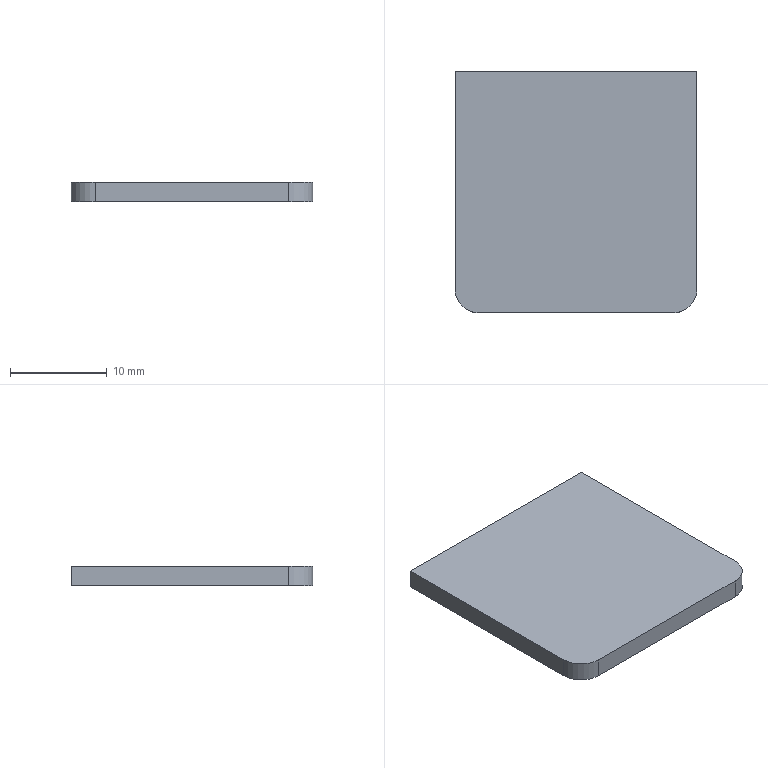Part | STEP file | 5090507 | 1 solid | 8 faces | box 25 x 25 x 2 mm | volume 1245 mm3 | plane 6 | cylinder 2 | commonest cylinder face diameters 5 x2
STEP:
#1=CARTESIAN_POINT('',(0.,0.,0.));
#2=DIRECTION('',(0.,0.,1.));
#3=DIRECTION('',(1.,0.,0.));
#4=AXIS2_PLACEMENT_3D('',#1,#2,#3);
#5=CARTESIAN_POINT('',(-12.5,12.5,0.));
#6=VERTEX_POINT('',#5);
#7=CARTESIAN_POINT('',(-12.5,-10.,0.));
#8=VERTEX_POINT('',#7);
#9=CARTESIAN_POINT('',(-12.5,12.5,0.));
#10=DIRECTION('',(0.,-1.,0.));
#11=VECTOR('',#10,1.);
#12=LINE('',#9,#11);
#13=CARTESIAN_POINT('',(-12.5,12.5,2.));
#14=DIRECTION('',(1.,0.,0.));
#15=DIRECTION('',(0.,1.,0.));
#16=AXIS2_PLACEMENT_3D('',#13,#14,#15);
#17=PLANE('',#16);
#18=CARTESIAN_POINT('',(0.,-2.));
#19=DIRECTION('',(-1.,0.));
#20=VECTOR('',#19,1.);
#21=LINE('',#18,#20);
#22=(GEOMETRIC_REPRESENTATION_CONTEXT(2)PARAMETRIC_REPRESENTATION_CONTEXT()REPRESENTATION_CONTEXT('',''));
#23=DEFINITIONAL_REPRESENTATION('',(#21),#22);
#24=PCURVE('',#17,#23);
#25=CARTESIAN_POINT('',(-10.,-10.,0.));
#26=DIRECTION('',(0.,0.,-1.));
#27=DIRECTION('',(-1.,0.,0.));
#28=AXIS2_PLACEMENT_3D('',#25,#26,#27);
#29=PLANE('',#28);
#30=CARTESIAN_POINT('',(2.5,22.5));
#31=DIRECTION('',(0.,-1.));
#32=VECTOR('',#31,1.);
#33=LINE('',#30,#32);
#34=(GEOMETRIC_REPRESENTATION_CONTEXT(2)PARAMETRIC_REPRESENTATION_CONTEXT()REPRESENTATION_CONTEXT('',''));
#35=DEFINITIONAL_REPRESENTATION('',(#33),#34);
#36=PCURVE('',#29,#35);
#37=SURFACE_CURVE('',#12,(#24,#36),.PCURVE_S1.);
#38=EDGE_CURVE('',#6,#8,#37,.T.);
#39=ORIENTED_EDGE('',*,*,#38,.T.);
#40=CARTESIAN_POINT('',(-12.5,-10.,2.));
#41=VERTEX_POINT('',#40);
#42=CARTESIAN_POINT('',(-12.5,-10.,2.));
#43=DIRECTION('',(0.,0.,-1.));
#44=VECTOR('',#43,1.);
#45=LINE('',#42,#44);
#46=CARTESIAN_POINT('',(-22.5,0.));
#47=DIRECTION('',(0.,-1.));
#48=VECTOR('',#47,1.);
#49=LINE('',#46,#48);
#50=(GEOMETRIC_REPRESENTATION_CONTEXT(2)PARAMETRIC_REPRESENTATION_CONTEXT()REPRESENTATION_CONTEXT('',''));
#51=DEFINITIONAL_REPRESENTATION('',(#49),#50);
#52=PCURVE('',#17,#51);
#53=CARTESIAN_POINT('',(-10.,-10.,2.));
#54=DIRECTION('',(0.,0.,-1.));
#55=DIRECTION('',(-1.,0.,0.));
#56=AXIS2_PLACEMENT_3D('',#53,#54,#55);
#57=CYLINDRICAL_SURFACE('',#56,2.5);
#58=CARTESIAN_POINT('',(6.283,0.));
#59=DIRECTION('',(0.,1.));
#60=VECTOR('',#59,1.);
#61=LINE('',#58,#60);
#62=(GEOMETRIC_REPRESENTATION_CONTEXT(2)PARAMETRIC_REPRESENTATION_CONTEXT()REPRESENTATION_CONTEXT('',''));
#63=DEFINITIONAL_REPRESENTATION('',(#61),#62);
#64=PCURVE('',#57,#63);
#65=SURFACE_CURVE('',#45,(#52,#64),.PCURVE_S1.);
#66=EDGE_CURVE('',#41,#8,#65,.T.);
#67=ORIENTED_EDGE('',*,*,#66,.F.);
#68=CARTESIAN_POINT('',(-12.5,12.5,2.));
#69=VERTEX_POINT('',#68);
#70=CARTESIAN_POINT('',(-12.5,12.5,2.));
#71=DIRECTION('',(0.,-1.,0.));
#72=VECTOR('',#71,1.);
#73=LINE('',#70,#72);
#74=CARTESIAN_POINT('',(0.,0.));
#75=DIRECTION('',(-1.,0.));
#76=VECTOR('',#75,1.);
#77=LINE('',#74,#76);
#78=(GEOMETRIC_REPRESENTATION_CONTEXT(2)PARAMETRIC_REPRESENTATION_CONTEXT()REPRESENTATION_CONTEXT('',''));
#79=DEFINITIONAL_REPRESENTATION('',(#77),#78);
#80=PCURVE('',#17,#79);
#81=CARTESIAN_POINT('',(-10.,-10.,2.));
#82=DIRECTION('',(0.,0.,-1.));
#83=DIRECTION('',(-1.,0.,0.));
#84=AXIS2_PLACEMENT_3D('',#81,#82,#83);
#85=PLANE('',#84);
#86=CARTESIAN_POINT('',(2.5,22.5));
#87=DIRECTION('',(0.,-1.));
#88=VECTOR('',#87,1.);
#89=LINE('',#86,#88);
#90=(GEOMETRIC_REPRESENTATION_CONTEXT(2)PARAMETRIC_REPRESENTATION_CONTEXT()REPRESENTATION_CONTEXT('',''));
#91=DEFINITIONAL_REPRESENTATION('',(#89),#90);
#92=PCURVE('',#85,#91);
#93=SURFACE_CURVE('',#73,(#80,#92),.PCURVE_S1.);
#94=EDGE_CURVE('',#69,#41,#93,.T.);
#95=ORIENTED_EDGE('',*,*,#94,.F.);
#96=CARTESIAN_POINT('',(-12.5,12.5,2.));
#97=DIRECTION('',(0.,0.,-1.));
#98=VECTOR('',#97,1.);
#99=LINE('',#96,#98);
#100=CARTESIAN_POINT('',(0.,0.));
#101=DIRECTION('',(0.,-1.));
#102=VECTOR('',#101,1.);
#103=LINE('',#100,#102);
#104=(GEOMETRIC_REPRESENTATION_CONTEXT(2)PARAMETRIC_REPRESENTATION_CONTEXT()REPRESENTATION_CONTEXT('',''));
#105=DEFINITIONAL_REPRESENTATION('',(#103),#104);
#106=PCURVE('',#17,#105);
#107=CARTESIAN_POINT('',(-12.5,12.5,2.));
#108=DIRECTION('',(0.,-1.,0.));
#109=DIRECTION('',(0.,0.,-1.));
#110=AXIS2_PLACEMENT_3D('',#107,#108,#109);
#111=PLANE('',#110);
#112=CARTESIAN_POINT('',(0.,0.));
#113=DIRECTION('',(1.,0.));
#114=VECTOR('',#113,1.);
#115=LINE('',#112,#114);
#116=(GEOMETRIC_REPRESENTATION_CONTEXT(2)PARAMETRIC_REPRESENTATION_CONTEXT()REPRESENTATION_CONTEXT('',''));
#117=DEFINITIONAL_REPRESENTATION('',(#115),#116);
#118=PCURVE('',#111,#117);
#119=SURFACE_CURVE('',#99,(#106,#118),.PCURVE_S1.);
#120=EDGE_CURVE('',#69,#6,#119,.T.);
#121=ORIENTED_EDGE('',*,*,#120,.T.);
#122=EDGE_LOOP('',(#39,#67,#95,#121));
#123=FACE_BOUND('',#122,.T.);
#124=ADVANCED_FACE('',(#123),#17,.F.);
#125=CARTESIAN_POINT('',(-10.,-12.5,0.));
#126=VERTEX_POINT('',#125);
#127=CARTESIAN_POINT('',(-10.,-10.,0.));
#128=DIRECTION('',(0.,0.,1.));
#129=DIRECTION('',(-1.,0.,0.));
#130=AXIS2_PLACEMENT_3D('',#127,#128,#129);
#131=CIRCLE('',#130,2.5);
#132=CARTESIAN_POINT('',(6.283,2.));
#133=DIRECTION('',(-1.,0.));
#134=VECTOR('',#133,1.);
#135=LINE('',#132,#134);
#136=(GEOMETRIC_REPRESENTATION_CONTEXT(2)PARAMETRIC_REPRESENTATION_CONTEXT()REPRESENTATION_CONTEXT('',''));
#137=DEFINITIONAL_REPRESENTATION('',(#135),#136);
#138=PCURVE('',#57,#137);
#139=CARTESIAN_POINT('',(2.5,0.));
#140=CARTESIAN_POINT('',(2.5,-4.33));
#141=CARTESIAN_POINT('',(-1.25,-2.165));
#142=CARTESIAN_POINT('',(-5.,0.));
#143=CARTESIAN_POINT('',(-1.25,2.165));
#144=CARTESIAN_POINT('',(2.5,4.33));
#145=CARTESIAN_POINT('',(2.5,0.));
#146=(BOUNDED_CURVE()B_SPLINE_CURVE(2,(#139,#140,#141,#142,#143,#144,#145),.UNSPECIFIED.,.T.,.F.)B_SPLINE_CURVE_WITH_KNOTS((1,2,2,2,2,1),(-2.094,0.,2.094,4.189,6.283,8.378),.UNSPECIFIED.)CURVE()GEOMETRIC_REPRESENTATION_ITEM()RATIONAL_B_SPLINE_CURVE((1.,0.5,1.,0.5,1.,0.5,1.))REPRESENTATION_ITEM(''));
#147=(GEOMETRIC_REPRESENTATION_CONTEXT(2)PARAMETRIC_REPRESENTATION_CONTEXT()REPRESENTATION_CONTEXT('',''));
#148=DEFINITIONAL_REPRESENTATION('',(#146),#147);
#149=PCURVE('',#29,#148);
#150=SURFACE_CURVE('',#131,(#138,#149),.PCURVE_S1.);
#151=EDGE_CURVE('',#8,#126,#150,.T.);
#152=ORIENTED_EDGE('',*,*,#151,.T.);
#153=CARTESIAN_POINT('',(-10.,-12.5,2.));
#154=VERTEX_POINT('',#153);
#155=CARTESIAN_POINT('',(-10.,-12.5,2.));
#156=DIRECTION('',(0.,0.,-1.));
#157=VECTOR('',#156,1.);
#158=LINE('',#155,#157);
#159=CARTESIAN_POINT('',(4.712,0.));
#160=DIRECTION('',(0.,1.));
#161=VECTOR('',#160,1.);
#162=LINE('',#159,#161);
#163=(GEOMETRIC_REPRESENTATION_CONTEXT(2)PARAMETRIC_REPRESENTATION_CONTEXT()REPRESENTATION_CONTEXT('',''));
#164=DEFINITIONAL_REPRESENTATION('',(#162),#163);
#165=PCURVE('',#57,#164);
#166=CARTESIAN_POINT('',(-10.,-12.5,2.));
#167=DIRECTION('',(0.,1.,0.));
#168=DIRECTION('',(0.,0.,1.));
#169=AXIS2_PLACEMENT_3D('',#166,#167,#168);
#170=PLANE('',#169);
#171=CARTESIAN_POINT('',(0.,0.));
#172=DIRECTION('',(-1.,0.));
#173=VECTOR('',#172,1.);
#174=LINE('',#171,#173);
#175=(GEOMETRIC_REPRESENTATION_CONTEXT(2)PARAMETRIC_REPRESENTATION_CONTEXT()REPRESENTATION_CONTEXT('',''));
#176=DEFINITIONAL_REPRESENTATION('',(#174),#175);
#177=PCURVE('',#170,#176);
#178=SURFACE_CURVE('',#158,(#165,#177),.PCURVE_S1.);
#179=EDGE_CURVE('',#154,#126,#178,.T.);
#180=ORIENTED_EDGE('',*,*,#179,.F.);
#181=CARTESIAN_POINT('',(-10.,-10.,2.));
#182=DIRECTION('',(0.,0.,1.));
#183=DIRECTION('',(-1.,0.,0.));
#184=AXIS2_PLACEMENT_3D('',#181,#182,#183);
#185=CIRCLE('',#184,2.5);
#186=CARTESIAN_POINT('',(6.283,0.));
#187=DIRECTION('',(-1.,0.));
#188=VECTOR('',#187,1.);
#189=LINE('',#186,#188);
#190=(GEOMETRIC_REPRESENTATION_CONTEXT(2)PARAMETRIC_REPRESENTATION_CONTEXT()REPRESENTATION_CONTEXT('',''));
#191=DEFINITIONAL_REPRESENTATION('',(#189),#190);
#192=PCURVE('',#57,#191);
#193=CARTESIAN_POINT('',(2.5,0.));
#194=CARTESIAN_POINT('',(2.5,-4.33));
#195=CARTESIAN_POINT('',(-1.25,-2.165));
#196=CARTESIAN_POINT('',(-5.,0.));
#197=CARTESIAN_POINT('',(-1.25,2.165));
#198=CARTESIAN_POINT('',(2.5,4.33));
#199=CARTESIAN_POINT('',(2.5,0.));
#200=(BOUNDED_CURVE()B_SPLINE_CURVE(2,(#193,#194,#195,#196,#197,#198,#199),.UNSPECIFIED.,.T.,.F.)B_SPLINE_CURVE_WITH_KNOTS((1,2,2,2,2,1),(-2.094,0.,2.094,4.189,6.283,8.378),.UNSPECIFIED.)CURVE()GEOMETRIC_REPRESENTATION_ITEM()RATIONAL_B_SPLINE_CURVE((1.,0.5,1.,0.5,1.,0.5,1.))REPRESENTATION_ITEM(''));
#201=(GEOMETRIC_REPRESENTATION_CONTEXT(2)PARAMETRIC_REPRESENTATION_CONTEXT()REPRESENTATION_CONTEXT('',''));
#202=DEFINITIONAL_REPRESENTATION('',(#200),#201);
#203=PCURVE('',#85,#202);
#204=SURFACE_CURVE('',#185,(#192,#203),.PCURVE_S1.);
#205=EDGE_CURVE('',#41,#154,#204,.T.);
#206=ORIENTED_EDGE('',*,*,#205,.F.);
#207=ORIENTED_EDGE('',*,*,#66,.T.);
#208=EDGE_LOOP('',(#152,#180,#206,#207));
#209=FACE_BOUND('',#208,.T.);
#210=ADVANCED_FACE('',(#209),#57,.T.);
#211=CARTESIAN_POINT('',(10.,-12.5,0.));
#212=VERTEX_POINT('',#211);
#213=CARTESIAN_POINT('',(-10.,-12.5,0.));
#214=DIRECTION('',(1.,0.,0.));
#215=VECTOR('',#214,1.);
#216=LINE('',#213,#215);
#217=CARTESIAN_POINT('',(-2.,0.));
#218=DIRECTION('',(0.,1.));
#219=VECTOR('',#218,1.);
#220=LINE('',#217,#219);
#221=(GEOMETRIC_REPRESENTATION_CONTEXT(2)PARAMETRIC_REPRESENTATION_CONTEXT()REPRESENTATION_CONTEXT('',''));
#222=DEFINITIONAL_REPRESENTATION('',(#220),#221);
#223=PCURVE('',#170,#222);
#224=CARTESIAN_POINT('',(0.,-2.5));
#225=DIRECTION('',(-1.,0.));
#226=VECTOR('',#225,1.);
#227=LINE('',#224,#226);
#228=(GEOMETRIC_REPRESENTATION_CONTEXT(2)PARAMETRIC_REPRESENTATION_CONTEXT()REPRESENTATION_CONTEXT('',''));
#229=DEFINITIONAL_REPRESENTATION('',(#227),#228);
#230=PCURVE('',#29,#229);
#231=SURFACE_CURVE('',#216,(#223,#230),.PCURVE_S1.);
#232=EDGE_CURVE('',#126,#212,#231,.T.);
#233=ORIENTED_EDGE('',*,*,#232,.T.);
#234=CARTESIAN_POINT('',(10.,-12.5,2.));
#235=VERTEX_POINT('',#234);
#236=CARTESIAN_POINT('',(10.,-12.5,2.));
#237=DIRECTION('',(0.,0.,-1.));
#238=VECTOR('',#237,1.);
#239=LINE('',#236,#238);
#240=CARTESIAN_POINT('',(0.,20.));
#241=DIRECTION('',(-1.,0.));
#242=VECTOR('',#241,1.);
#243=LINE('',#240,#242);
#244=(GEOMETRIC_REPRESENTATION_CONTEXT(2)PARAMETRIC_REPRESENTATION_CONTEXT()REPRESENTATION_CONTEXT('',''));
#245=DEFINITIONAL_REPRESENTATION('',(#243),#244);
#246=PCURVE('',#170,#245);
#247=CARTESIAN_POINT('',(10.,-10.,2.));
#248=DIRECTION('',(0.,0.,-1.));
#249=DIRECTION('',(-1.,0.,0.));
#250=AXIS2_PLACEMENT_3D('',#247,#248,#249);
#251=CYLINDRICAL_SURFACE('',#250,2.5);
#252=CARTESIAN_POINT('',(4.712,0.));
#253=DIRECTION('',(0.,1.));
#254=VECTOR('',#253,1.);
#255=LINE('',#252,#254);
#256=(GEOMETRIC_REPRESENTATION_CONTEXT(2)PARAMETRIC_REPRESENTATION_CONTEXT()REPRESENTATION_CONTEXT('',''));
#257=DEFINITIONAL_REPRESENTATION('',(#255),#256);
#258=PCURVE('',#251,#257);
#259=SURFACE_CURVE('',#239,(#246,#258),.PCURVE_S1.);
#260=EDGE_CURVE('',#235,#212,#259,.T.);
#261=ORIENTED_EDGE('',*,*,#260,.F.);
#262=CARTESIAN_POINT('',(-10.,-12.5,2.));
#263=DIRECTION('',(1.,0.,0.));
#264=VECTOR('',#263,1.);
#265=LINE('',#262,#264);
#266=CARTESIAN_POINT('',(0.,0.));
#267=DIRECTION('',(0.,1.));
#268=VECTOR('',#267,1.);
#269=LINE('',#266,#268);
#270=(GEOMETRIC_REPRESENTATION_CONTEXT(2)PARAMETRIC_REPRESENTATION_CONTEXT()REPRESENTATION_CONTEXT('',''));
#271=DEFINITIONAL_REPRESENTATION('',(#269),#270);
#272=PCURVE('',#170,#271);
#273=CARTESIAN_POINT('',(0.,-2.5));
#274=DIRECTION('',(-1.,0.));
#275=VECTOR('',#274,1.);
#276=LINE('',#273,#275);
#277=(GEOMETRIC_REPRESENTATION_CONTEXT(2)PARAMETRIC_REPRESENTATION_CONTEXT()REPRESENTATION_CONTEXT('',''));
#278=DEFINITIONAL_REPRESENTATION('',(#276),#277);
#279=PCURVE('',#85,#278);
#280=SURFACE_CURVE('',#265,(#272,#279),.PCURVE_S1.);
#281=EDGE_CURVE('',#154,#235,#280,.T.);
#282=ORIENTED_EDGE('',*,*,#281,.F.);
#283=ORIENTED_EDGE('',*,*,#179,.T.);
#284=EDGE_LOOP('',(#233,#261,#282,#283));
#285=FACE_BOUND('',#284,.T.);
#286=ADVANCED_FACE('',(#285),#170,.F.);
#287=CARTESIAN_POINT('',(12.5,-10.,0.));
#288=VERTEX_POINT('',#287);
#289=CARTESIAN_POINT('',(10.,-10.,0.));
#290=DIRECTION('',(0.,0.,1.));
#291=DIRECTION('',(-1.,0.,0.));
#292=AXIS2_PLACEMENT_3D('',#289,#290,#291);
#293=CIRCLE('',#292,2.5);
#294=CARTESIAN_POINT('',(6.283,2.));
#295=DIRECTION('',(-1.,0.));
#296=VECTOR('',#295,1.);
#297=LINE('',#294,#296);
#298=(GEOMETRIC_REPRESENTATION_CONTEXT(2)PARAMETRIC_REPRESENTATION_CONTEXT()REPRESENTATION_CONTEXT('',''));
#299=DEFINITIONAL_REPRESENTATION('',(#297),#298);
#300=PCURVE('',#251,#299);
#301=CARTESIAN_POINT('',(-17.5,0.));
#302=CARTESIAN_POINT('',(-17.5,-4.33));
#303=CARTESIAN_POINT('',(-21.25,-2.165));
#304=CARTESIAN_POINT('',(-25.,0.));
#305=CARTESIAN_POINT('',(-21.25,2.165));
#306=CARTESIAN_POINT('',(-17.5,4.33));
#307=CARTESIAN_POINT('',(-17.5,0.));
#308=(BOUNDED_CURVE()B_SPLINE_CURVE(2,(#301,#302,#303,#304,#305,#306,#307),.UNSPECIFIED.,.T.,.F.)B_SPLINE_CURVE_WITH_KNOTS((1,2,2,2,2,1),(-2.094,0.,2.094,4.189,6.283,8.378),.UNSPECIFIED.)CURVE()GEOMETRIC_REPRESENTATION_ITEM()RATIONAL_B_SPLINE_CURVE((1.,0.5,1.,0.5,1.,0.5,1.))REPRESENTATION_ITEM(''));
#309=(GEOMETRIC_REPRESENTATION_CONTEXT(2)PARAMETRIC_REPRESENTATION_CONTEXT()REPRESENTATION_CONTEXT('',''));
#310=DEFINITIONAL_REPRESENTATION('',(#308),#309);
#311=PCURVE('',#29,#310);
#312=SURFACE_CURVE('',#293,(#300,#311),.PCURVE_S1.);
#313=EDGE_CURVE('',#212,#288,#312,.T.);
#314=ORIENTED_EDGE('',*,*,#313,.T.);
#315=CARTESIAN_POINT('',(12.5,-10.,2.));
#316=VERTEX_POINT('',#315);
#317=CARTESIAN_POINT('',(12.5,-10.,2.));
#318=DIRECTION('',(0.,0.,-1.));
#319=VECTOR('',#318,1.);
#320=LINE('',#317,#319);
#321=CARTESIAN_POINT('',(3.142,0.));
#322=DIRECTION('',(0.,1.));
#323=VECTOR('',#322,1.);
#324=LINE('',#321,#323);
#325=(GEOMETRIC_REPRESENTATION_CONTEXT(2)PARAMETRIC_REPRESENTATION_CONTEXT()REPRESENTATION_CONTEXT('',''));
#326=DEFINITIONAL_REPRESENTATION('',(#324),#325);
#327=PCURVE('',#251,#326);
#328=CARTESIAN_POINT('',(12.5,12.5,2.));
#329=DIRECTION('',(-1.,0.,0.));
#330=DIRECTION('',(0.,-1.,0.));
#331=AXIS2_PLACEMENT_3D('',#328,#329,#330);
#332=PLANE('',#331);
#333=CARTESIAN_POINT('',(22.5,0.));
#334=DIRECTION('',(0.,-1.));
#335=VECTOR('',#334,1.);
#336=LINE('',#333,#335);
#337=(GEOMETRIC_REPRESENTATION_CONTEXT(2)PARAMETRIC_REPRESENTATION_CONTEXT()REPRESENTATION_CONTEXT('',''));
#338=DEFINITIONAL_REPRESENTATION('',(#336),#337);
#339=PCURVE('',#332,#338);
#340=SURFACE_CURVE('',#320,(#327,#339),.PCURVE_S1.);
#341=EDGE_CURVE('',#316,#288,#340,.T.);
#342=ORIENTED_EDGE('',*,*,#341,.F.);
#343=CARTESIAN_POINT('',(10.,-10.,2.));
#344=DIRECTION('',(0.,0.,1.));
#345=DIRECTION('',(-1.,0.,0.));
#346=AXIS2_PLACEMENT_3D('',#343,#344,#345);
#347=CIRCLE('',#346,2.5);
#348=CARTESIAN_POINT('',(6.283,0.));
#349=DIRECTION('',(-1.,0.));
#350=VECTOR('',#349,1.);
#351=LINE('',#348,#350);
#352=(GEOMETRIC_REPRESENTATION_CONTEXT(2)PARAMETRIC_REPRESENTATION_CONTEXT()REPRESENTATION_CONTEXT('',''));
#353=DEFINITIONAL_REPRESENTATION('',(#351),#352);
#354=PCURVE('',#251,#353);
#355=CARTESIAN_POINT('',(-17.5,0.));
#356=CARTESIAN_POINT('',(-17.5,-4.33));
#357=CARTESIAN_POINT('',(-21.25,-2.165));
#358=CARTESIAN_POINT('',(-25.,0.));
#359=CARTESIAN_POINT('',(-21.25,2.165));
#360=CARTESIAN_POINT('',(-17.5,4.33));
#361=CARTESIAN_POINT('',(-17.5,0.));
#362=(BOUNDED_CURVE()B_SPLINE_CURVE(2,(#355,#356,#357,#358,#359,#360,#361),.UNSPECIFIED.,.T.,.F.)B_SPLINE_CURVE_WITH_KNOTS((1,2,2,2,2,1),(-2.094,0.,2.094,4.189,6.283,8.378),.UNSPECIFIED.)CURVE()GEOMETRIC_REPRESENTATION_ITEM()RATIONAL_B_SPLINE_CURVE((1.,0.5,1.,0.5,1.,0.5,1.))REPRESENTATION_ITEM(''));
#363=(GEOMETRIC_REPRESENTATION_CONTEXT(2)PARAMETRIC_REPRESENTATION_CONTEXT()REPRESENTATION_CONTEXT('',''));
#364=DEFINITIONAL_REPRESENTATION('',(#362),#363);
#365=PCURVE('',#85,#364);
#366=SURFACE_CURVE('',#347,(#354,#365),.PCURVE_S1.);
#367=EDGE_CURVE('',#235,#316,#366,.T.);
#368=ORIENTED_EDGE('',*,*,#367,.F.);
#369=ORIENTED_EDGE('',*,*,#260,.T.);
#370=EDGE_LOOP('',(#314,#342,#368,#369));
#371=FACE_BOUND('',#370,.T.);
#372=ADVANCED_FACE('',(#371),#251,.T.);
#373=CARTESIAN_POINT('',(12.5,12.5,0.));
#374=VERTEX_POINT('',#373);
#375=CARTESIAN_POINT('',(12.5,12.5,0.));
#376=DIRECTION('',(0.,1.,0.));
#377=VECTOR('',#376,1.);
#378=LINE('',#375,#377);
#379=CARTESIAN_POINT('',(0.,-2.));
#380=DIRECTION('',(-1.,0.));
#381=VECTOR('',#380,1.);
#382=LINE('',#379,#381);
#383=(GEOMETRIC_REPRESENTATION_CONTEXT(2)PARAMETRIC_REPRESENTATION_CONTEXT()REPRESENTATION_CONTEXT('',''));
#384=DEFINITIONAL_REPRESENTATION('',(#382),#383);
#385=PCURVE('',#332,#384);
#386=CARTESIAN_POINT('',(-22.5,22.5));
#387=DIRECTION('',(0.,1.));
#388=VECTOR('',#387,1.);
#389=LINE('',#386,#388);
#390=(GEOMETRIC_REPRESENTATION_CONTEXT(2)PARAMETRIC_REPRESENTATION_CONTEXT()REPRESENTATION_CONTEXT('',''));
#391=DEFINITIONAL_REPRESENTATION('',(#389),#390);
#392=PCURVE('',#29,#391);
#393=SURFACE_CURVE('',#378,(#385,#392),.PCURVE_S1.);
#394=EDGE_CURVE('',#288,#374,#393,.T.);
#395=ORIENTED_EDGE('',*,*,#394,.T.);
#396=CARTESIAN_POINT('',(12.5,12.5,2.));
#397=VERTEX_POINT('',#396);
#398=CARTESIAN_POINT('',(12.5,12.5,2.));
#399=DIRECTION('',(0.,0.,-1.));
#400=VECTOR('',#399,1.);
#401=LINE('',#398,#400);
#402=CARTESIAN_POINT('',(0.,0.));
#403=DIRECTION('',(0.,-1.));
#404=VECTOR('',#403,1.);
#405=LINE('',#402,#404);
#406=(GEOMETRIC_REPRESENTATION_CONTEXT(2)PARAMETRIC_REPRESENTATION_CONTEXT()REPRESENTATION_CONTEXT('',''));
#407=DEFINITIONAL_REPRESENTATION('',(#405),#406);
#408=PCURVE('',#332,#407);
#409=CARTESIAN_POINT('',(0.,25.));
#410=DIRECTION('',(1.,0.));
#411=VECTOR('',#410,1.);
#412=LINE('',#409,#411);
#413=(GEOMETRIC_REPRESENTATION_CONTEXT(2)PARAMETRIC_REPRESENTATION_CONTEXT()REPRESENTATION_CONTEXT('',''));
#414=DEFINITIONAL_REPRESENTATION('',(#412),#413);
#415=PCURVE('',#111,#414);
#416=SURFACE_CURVE('',#401,(#408,#415),.PCURVE_S1.);
#417=EDGE_CURVE('',#397,#374,#416,.T.);
#418=ORIENTED_EDGE('',*,*,#417,.F.);
#419=CARTESIAN_POINT('',(12.5,12.5,2.));
#420=DIRECTION('',(0.,1.,0.));
#421=VECTOR('',#420,1.);
#422=LINE('',#419,#421);
#423=CARTESIAN_POINT('',(0.,0.));
#424=DIRECTION('',(-1.,0.));
#425=VECTOR('',#424,1.);
#426=LINE('',#423,#425);
#427=(GEOMETRIC_REPRESENTATION_CONTEXT(2)PARAMETRIC_REPRESENTATION_CONTEXT()REPRESENTATION_CONTEXT('',''));
#428=DEFINITIONAL_REPRESENTATION('',(#426),#427);
#429=PCURVE('',#332,#428);
#430=CARTESIAN_POINT('',(-22.5,22.5));
#431=DIRECTION('',(0.,1.));
#432=VECTOR('',#431,1.);
#433=LINE('',#430,#432);
#434=(GEOMETRIC_REPRESENTATION_CONTEXT(2)PARAMETRIC_REPRESENTATION_CONTEXT()REPRESENTATION_CONTEXT('',''));
#435=DEFINITIONAL_REPRESENTATION('',(#433),#434);
#436=PCURVE('',#85,#435);
#437=SURFACE_CURVE('',#422,(#429,#436),.PCURVE_S1.);
#438=EDGE_CURVE('',#316,#397,#437,.T.);
#439=ORIENTED_EDGE('',*,*,#438,.F.);
#440=ORIENTED_EDGE('',*,*,#341,.T.);
#441=EDGE_LOOP('',(#395,#418,#439,#440));
#442=FACE_BOUND('',#441,.T.);
#443=ADVANCED_FACE('',(#442),#332,.F.);
#444=CARTESIAN_POINT('',(-12.5,12.5,0.));
#445=DIRECTION('',(-1.,0.,0.));
#446=VECTOR('',#445,1.);
#447=LINE('',#444,#446);
#448=CARTESIAN_POINT('',(2.,0.));
#449=DIRECTION('',(0.,-1.));
#450=VECTOR('',#449,1.);
#451=LINE('',#448,#450);
#452=(GEOMETRIC_REPRESENTATION_CONTEXT(2)PARAMETRIC_REPRESENTATION_CONTEXT()REPRESENTATION_CONTEXT('',''));
#453=DEFINITIONAL_REPRESENTATION('',(#451),#452);
#454=PCURVE('',#111,#453);
#455=CARTESIAN_POINT('',(2.5,22.5));
#456=DIRECTION('',(1.,0.));
#457=VECTOR('',#456,1.);
#458=LINE('',#455,#457);
#459=(GEOMETRIC_REPRESENTATION_CONTEXT(2)PARAMETRIC_REPRESENTATION_CONTEXT()REPRESENTATION_CONTEXT('',''));
#460=DEFINITIONAL_REPRESENTATION('',(#458),#459);
#461=PCURVE('',#29,#460);
#462=SURFACE_CURVE('',#447,(#454,#461),.PCURVE_S1.);
#463=EDGE_CURVE('',#374,#6,#462,.T.);
#464=ORIENTED_EDGE('',*,*,#463,.T.);
#465=ORIENTED_EDGE('',*,*,#120,.F.);
#466=CARTESIAN_POINT('',(-12.5,12.5,2.));
#467=DIRECTION('',(-1.,0.,0.));
#468=VECTOR('',#467,1.);
#469=LINE('',#466,#468);
#470=CARTESIAN_POINT('',(0.,0.));
#471=DIRECTION('',(0.,-1.));
#472=VECTOR('',#471,1.);
#473=LINE('',#470,#472);
#474=(GEOMETRIC_REPRESENTATION_CONTEXT(2)PARAMETRIC_REPRESENTATION_CONTEXT()REPRESENTATION_CONTEXT('',''));
#475=DEFINITIONAL_REPRESENTATION('',(#473),#474);
#476=PCURVE('',#111,#475);
#477=CARTESIAN_POINT('',(2.5,22.5));
#478=DIRECTION('',(1.,0.));
#479=VECTOR('',#478,1.);
#480=LINE('',#477,#479);
#481=(GEOMETRIC_REPRESENTATION_CONTEXT(2)PARAMETRIC_REPRESENTATION_CONTEXT()REPRESENTATION_CONTEXT('',''));
#482=DEFINITIONAL_REPRESENTATION('',(#480),#481);
#483=PCURVE('',#85,#482);
#484=SURFACE_CURVE('',#469,(#476,#483),.PCURVE_S1.);
#485=EDGE_CURVE('',#397,#69,#484,.T.);
#486=ORIENTED_EDGE('',*,*,#485,.F.);
#487=ORIENTED_EDGE('',*,*,#417,.T.);
#488=EDGE_LOOP('',(#464,#465,#486,#487));
#489=FACE_BOUND('',#488,.T.);
#490=ADVANCED_FACE('',(#489),#111,.F.);
#491=ORIENTED_EDGE('',*,*,#94,.T.);
#492=ORIENTED_EDGE('',*,*,#205,.T.);
#493=ORIENTED_EDGE('',*,*,#281,.T.);
#494=ORIENTED_EDGE('',*,*,#367,.T.);
#495=ORIENTED_EDGE('',*,*,#438,.T.);
#496=ORIENTED_EDGE('',*,*,#485,.T.);
#497=EDGE_LOOP('',(#491,#492,#493,#494,#495,#496));
#498=FACE_BOUND('',#497,.T.);
#499=ADVANCED_FACE('',(#498),#85,.F.);
#500=ORIENTED_EDGE('',*,*,#38,.F.);
#501=ORIENTED_EDGE('',*,*,#463,.F.);
#502=ORIENTED_EDGE('',*,*,#394,.F.);
#503=ORIENTED_EDGE('',*,*,#313,.F.);
#504=ORIENTED_EDGE('',*,*,#232,.F.);
#505=ORIENTED_EDGE('',*,*,#151,.F.);
#506=EDGE_LOOP('',(#500,#501,#502,#503,#504,#505));
#507=FACE_BOUND('',#506,.T.);
#508=ADVANCED_FACE('',(#507),#29,.T.);
#509=CLOSED_SHELL('',(#124,#210,#286,#372,#443,#490,#499,#508));
#510=MANIFOLD_SOLID_BREP('',#509);
#511=(LENGTH_UNIT()NAMED_UNIT(*)SI_UNIT(.MILLI.,.METRE.));
#512=UNCERTAINTY_MEASURE_WITH_UNIT(LENGTH_MEASURE(0.0000001),#511,'','');
#513=(NAMED_UNIT(*)PLANE_ANGLE_UNIT()SI_UNIT($,.RADIAN.));
#514=(NAMED_UNIT(*)SI_UNIT($,.STERADIAN.)SOLID_ANGLE_UNIT());
#515=(GEOMETRIC_REPRESENTATION_CONTEXT(3)GLOBAL_UNCERTAINTY_ASSIGNED_CONTEXT((#512))GLOBAL_UNIT_ASSIGNED_CONTEXT((#511,#513,#514))REPRESENTATION_CONTEXT('',''));
#516=ADVANCED_BREP_SHAPE_REPRESENTATION('',(#4,#510),#515);